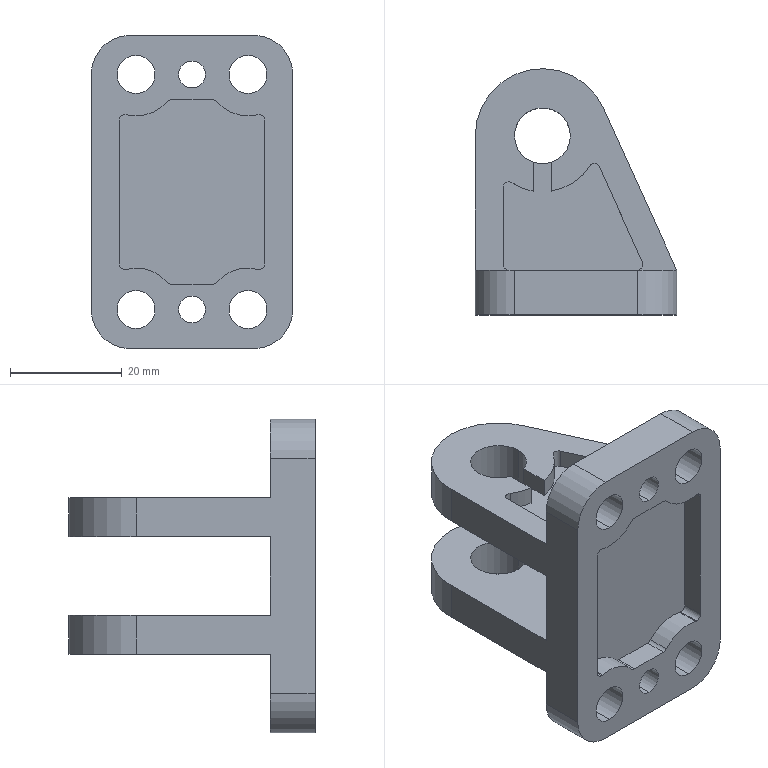Part | SolidWorks | features ICE 10, Fillet 2, HoleWzd 2, RevCut 2, Extrusion 1 | 1 solid | 80 faces | box 36 x 44 x 56 mm | volume 21149 mm3 | cylinder 51 | plane 29 | commonest cylinder face diameters 2 x19 6.8 x8 14.8 x6 4.8 x4 10 x4 14 x4